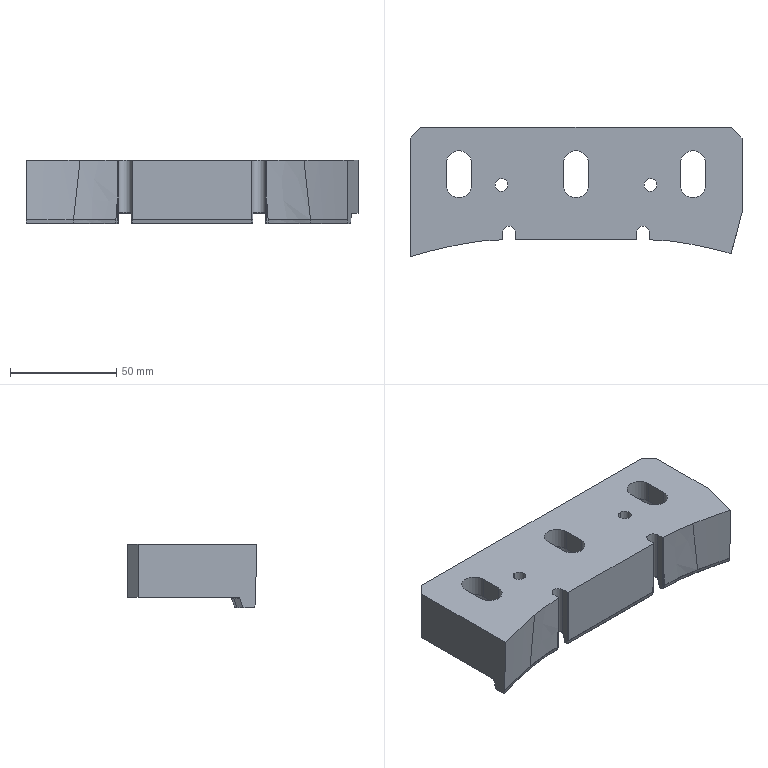NC program | Mastercam | posted with a generic post | part box 156 x 60.706 x 30 mm
Lines 1 to 36 of 78092:
%
O0000()
(MATERIAL - ALUMINUM MM - 2024)
( T1 | 63 FEM | H1 )
( T20 | 20 BNOS | H20 | XY STOCK TO LEAVE - .1 | Z STOCK TO LEAVE - 0. )
( T10 | 10 FEM | H10 | XY STOCK TO LEAVE - .1 | Z STOCK TO LEAVE - 0. )
( T11 | 10 FEM | H11 )
( T4 | 4 FEM | H4 | XY STOCK TO LEAVE - .1 | Z STOCK TO LEAVE - 0. )
( T14 | 4 FEM | H14 )
( T21 | 6 CHMI | H21 )
( T18 | 6 BNOS | H18 | XY STOCK TO LEAVE - .15 | Z STOCK TO LEAVE - 0. )
( T16 | 16 FEM | H16 | XY STOCK TO LEAVE - .1 | Z STOCK TO LEAVE - .05 )
( T6 | 6 FEM | H6 | XY STOCK TO LEAVE - .06 | Z STOCK TO LEAVE - 0. )
( T2 | 6 FEM | H2 )
N100 G21
N110 G0 G17 G40 G49 G80 G90
N120 T1 M6
N130 G0 G90 G54 X132.361 Y-26.23 A0. S800 M3
N140 G43 H1 Z50. M8
N150 Z10.
N160 G1 Z0. F600.
N170 X81.961 F300.
N180 X-81.206
N190 X-131.606
N200 G0 Z25.
N210 X132.361 Y3.77
N220 Z10.
N230 G1 Z0. F600.
N240 X81.961 F300.
N250 X-81.206
N260 X-131.606
N270 G0 Z50.
N280 M5
N290 G91 G28 Z0. M9
N300 A0.
N310 M01